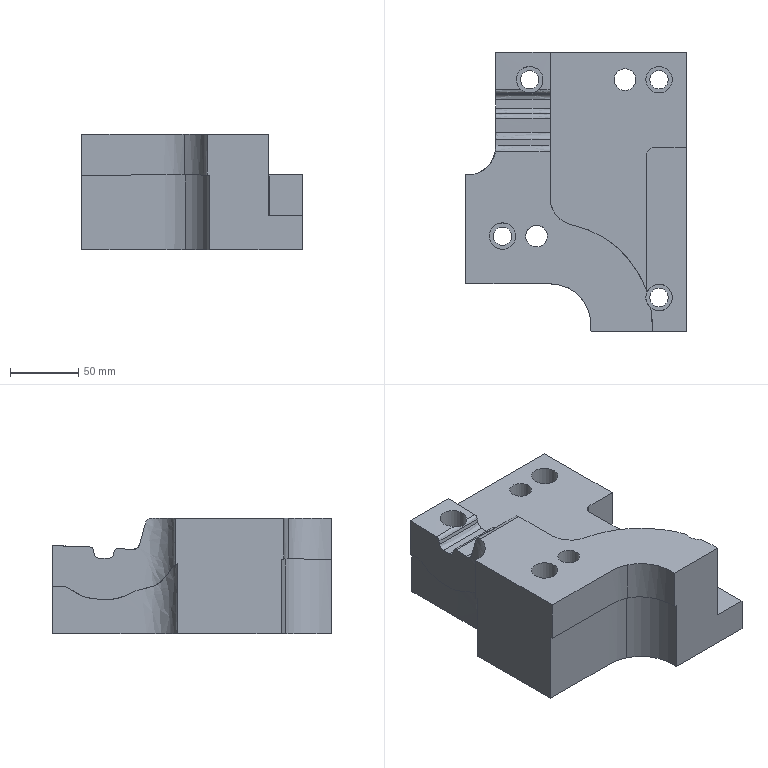Part | NX | features solid 2 | 1 solid | 50 faces | box 162 x 205 x 85 mm | volume 1650370 mm3 | spline 21 | plane 15 | cylinder 14 | commonest cylinder face diameters 13.5 x4 19.5 x4 16 x2 150 x2 10 x1 40 x1